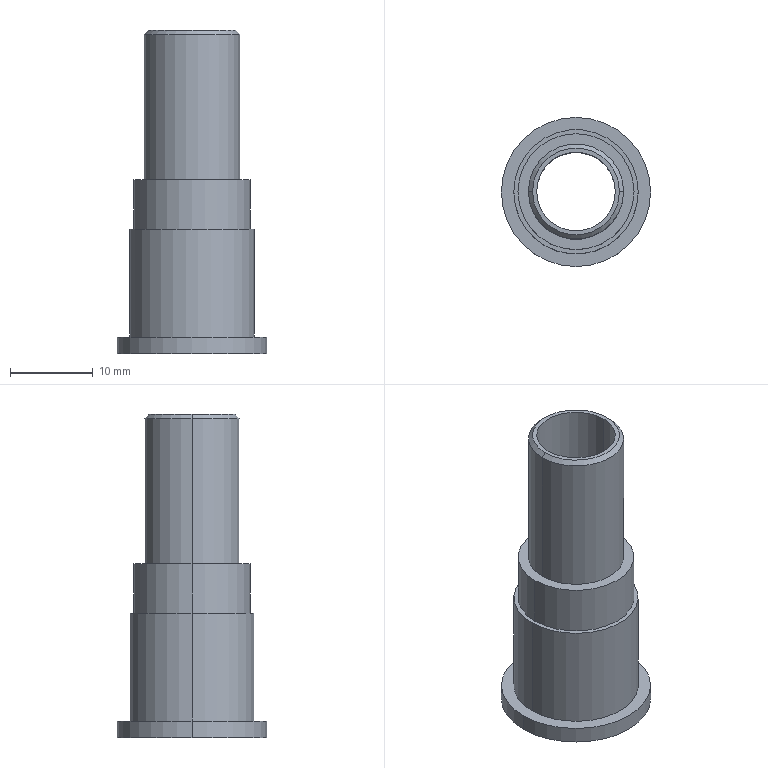Part | SolidWorks | features ICE 4, Chamfer 2, Extrusion 1 | 1 solid | 19 faces | box 18 x 18 x 39 mm | volume 2785 mm3 | cylinder 10 | plane 5 | cone 4 | commonest cylinder face diameters 9.5 x2 11.5 x2 14 x2 15 x2 18 x2
STEP:
#1=CARTESIAN_POINT('',(4.75,0.,10.));
#2=VERTEX_POINT('',#1);
#3=CARTESIAN_POINT('',(-4.75,0.,10.));
#4=VERTEX_POINT('',#3);
#5=CARTESIAN_POINT('',(0.,0.,10.));
#6=DIRECTION('',(0.,0.,-1.));
#7=DIRECTION('',(1.,0.,0.));
#8=AXIS2_PLACEMENT_3D('',#5,#6,#7);
#9=CIRCLE('',#8,4.75);
#10=EDGE_CURVE('',#2,#4,#9,.T.);
#11=ORIENTED_EDGE('',*,*,#10,.F.);
#12=CARTESIAN_POINT('',(5.05,0.,0.));
#13=VERTEX_POINT('',#12);
#14=CARTESIAN_POINT('',(4.75,0.,10.));
#15=DIRECTION('',(0.02999,0.,-0.9996));
#16=VECTOR('',#15,1000.);
#17=LINE('',#14,#16);
#18=EDGE_CURVE('',#2,#13,#17,.T.);
#19=ORIENTED_EDGE('',*,*,#18,.T.);
#20=CARTESIAN_POINT('',(-5.05,0.,0.));
#21=VERTEX_POINT('',#20);
#22=CARTESIAN_POINT('',(0.,0.,0.));
#23=DIRECTION('',(0.,0.,1.));
#24=DIRECTION('',(1.,0.,0.));
#25=AXIS2_PLACEMENT_3D('',#22,#23,#24);
#26=CIRCLE('',#25,5.05);
#27=EDGE_CURVE('',#21,#13,#26,.T.);
#28=ORIENTED_EDGE('',*,*,#27,.F.);
#29=CARTESIAN_POINT('',(-4.75,0.,10.));
#30=DIRECTION('',(-0.02999,0.,-0.9996));
#31=VECTOR('',#30,1000.);
#32=LINE('',#29,#31);
#33=EDGE_CURVE('',#4,#21,#32,.T.);
#34=ORIENTED_EDGE('',*,*,#33,.F.);
#35=EDGE_LOOP('',(#11,#19,#28,#34));
#36=FACE_OUTER_BOUND('',#35,.T.);
#37=CARTESIAN_POINT('',(0.,0.,10.));
#38=DIRECTION('',(0.,0.,-1.));
#39=DIRECTION('',(-1.,0.,0.));
#40=AXIS2_PLACEMENT_3D('',#37,#38,#39);
#41=CONICAL_SURFACE('',#40,4.75,0.02999);
#42=ADVANCED_FACE('',(#36),#41,.F.);
#43=CARTESIAN_POINT('',(5.25,0.,39.));
#44=VERTEX_POINT('',#43);
#45=CARTESIAN_POINT('',(-5.25,0.,39.));
#46=VERTEX_POINT('',#45);
#47=CARTESIAN_POINT('',(0.,0.,39.));
#48=DIRECTION('',(0.,0.,1.));
#49=DIRECTION('',(1.,0.,0.));
#50=AXIS2_PLACEMENT_3D('',#47,#48,#49);
#51=CIRCLE('',#50,5.25);
#52=EDGE_CURVE('',#44,#46,#51,.T.);
#53=ORIENTED_EDGE('',*,*,#52,.F.);
#54=CARTESIAN_POINT('',(5.75,0.,38.5));
#55=VERTEX_POINT('',#54);
#56=CARTESIAN_POINT('',(5.25,0.,39.));
#57=DIRECTION('',(0.7071,0.,-0.7071));
#58=VECTOR('',#57,1000.);
#59=LINE('',#56,#58);
#60=EDGE_CURVE('',#44,#55,#59,.T.);
#61=ORIENTED_EDGE('',*,*,#60,.T.);
#62=CARTESIAN_POINT('',(-5.75,0.,38.5));
#63=VERTEX_POINT('',#62);
#64=CARTESIAN_POINT('',(0.,0.,38.5));
#65=DIRECTION('',(0.,0.,-1.));
#66=DIRECTION('',(1.,0.,0.));
#67=AXIS2_PLACEMENT_3D('',#64,#65,#66);
#68=CIRCLE('',#67,5.75);
#69=EDGE_CURVE('',#63,#55,#68,.T.);
#70=ORIENTED_EDGE('',*,*,#69,.F.);
#71=CARTESIAN_POINT('',(-5.25,0.,39.));
#72=DIRECTION('',(-0.7071,0.,-0.7071));
#73=VECTOR('',#72,1000.);
#74=LINE('',#71,#73);
#75=EDGE_CURVE('',#46,#63,#74,.T.);
#76=ORIENTED_EDGE('',*,*,#75,.F.);
#77=EDGE_LOOP('',(#53,#61,#70,#76));
#78=FACE_OUTER_BOUND('',#77,.T.);
#79=CARTESIAN_POINT('',(0.,0.,39.));
#80=DIRECTION('',(0.,0.,-1.));
#81=DIRECTION('',(-1.,0.,0.));
#82=AXIS2_PLACEMENT_3D('',#79,#80,#81);
#83=CONICAL_SURFACE('',#82,5.25,0.7854);
#84=ADVANCED_FACE('',(#78),#83,.T.);
#85=CARTESIAN_POINT('',(4.75,0.,39.));
#86=VERTEX_POINT('',#85);
#87=CARTESIAN_POINT('',(-4.75,0.,39.));
#88=VERTEX_POINT('',#87);
#89=CARTESIAN_POINT('',(0.,0.,39.));
#90=DIRECTION('',(0.,0.,-1.));
#91=DIRECTION('',(-1.,0.,0.));
#92=AXIS2_PLACEMENT_3D('',#89,#90,#91);
#93=CIRCLE('',#92,4.75);
#94=EDGE_CURVE('',#86,#88,#93,.T.);
#95=ORIENTED_EDGE('',*,*,#94,.F.);
#96=CARTESIAN_POINT('',(4.75,0.,39.));
#97=DIRECTION('',(0.,0.,-1.));
#98=VECTOR('',#97,1000.);
#99=LINE('',#96,#98);
#100=EDGE_CURVE('',#86,#2,#99,.T.);
#101=ORIENTED_EDGE('',*,*,#100,.T.);
#102=ORIENTED_EDGE('',*,*,#10,.T.);
#103=CARTESIAN_POINT('',(-4.75,0.,39.));
#104=DIRECTION('',(0.,0.,-1.));
#105=VECTOR('',#104,1000.);
#106=LINE('',#103,#105);
#107=EDGE_CURVE('',#88,#4,#106,.T.);
#108=ORIENTED_EDGE('',*,*,#107,.F.);
#109=EDGE_LOOP('',(#95,#101,#102,#108));
#110=FACE_OUTER_BOUND('',#109,.T.);
#111=CARTESIAN_POINT('',(0.,0.,39.));
#112=DIRECTION('',(0.,0.,-1.));
#113=DIRECTION('',(-1.,0.,0.));
#114=AXIS2_PLACEMENT_3D('',#111,#112,#113);
#115=CYLINDRICAL_SURFACE('',#114,4.75);
#116=ADVANCED_FACE('',(#110),#115,.F.);
#117=ORIENTED_EDGE('',*,*,#69,.T.);
#118=CARTESIAN_POINT('',(5.75,0.,21.));
#119=VERTEX_POINT('',#118);
#120=CARTESIAN_POINT('',(5.75,0.,39.));
#121=DIRECTION('',(0.,0.,-1.));
#122=VECTOR('',#121,1000.);
#123=LINE('',#120,#122);
#124=EDGE_CURVE('',#55,#119,#123,.T.);
#125=ORIENTED_EDGE('',*,*,#124,.T.);
#126=CARTESIAN_POINT('',(-5.75,0.,21.));
#127=VERTEX_POINT('',#126);
#128=CARTESIAN_POINT('',(0.,0.,21.));
#129=DIRECTION('',(0.,0.,1.));
#130=DIRECTION('',(1.,0.,0.));
#131=AXIS2_PLACEMENT_3D('',#128,#129,#130);
#132=CIRCLE('',#131,5.75);
#133=EDGE_CURVE('',#119,#127,#132,.T.);
#134=ORIENTED_EDGE('',*,*,#133,.T.);
#135=CARTESIAN_POINT('',(-5.75,0.,39.));
#136=DIRECTION('',(0.,0.,-1.));
#137=VECTOR('',#136,1000.);
#138=LINE('',#135,#137);
#139=EDGE_CURVE('',#63,#127,#138,.T.);
#140=ORIENTED_EDGE('',*,*,#139,.F.);
#141=EDGE_LOOP('',(#117,#125,#134,#140));
#142=FACE_OUTER_BOUND('',#141,.T.);
#143=CARTESIAN_POINT('',(0.,0.,39.));
#144=DIRECTION('',(0.,0.,-1.));
#145=DIRECTION('',(-1.,0.,0.));
#146=AXIS2_PLACEMENT_3D('',#143,#144,#145);
#147=CYLINDRICAL_SURFACE('',#146,5.75);
#148=ADVANCED_FACE('',(#142),#147,.T.);
#149=CARTESIAN_POINT('',(7.,0.,21.));
#150=VERTEX_POINT('',#149);
#151=CARTESIAN_POINT('',(-7.,0.,21.));
#152=VERTEX_POINT('',#151);
#153=CARTESIAN_POINT('',(0.,0.,21.));
#154=DIRECTION('',(0.,0.,1.));
#155=DIRECTION('',(1.,0.,0.));
#156=AXIS2_PLACEMENT_3D('',#153,#154,#155);
#157=CIRCLE('',#156,7.);
#158=EDGE_CURVE('',#150,#152,#157,.T.);
#159=ORIENTED_EDGE('',*,*,#158,.F.);
#160=CARTESIAN_POINT('',(7.,0.,15.));
#161=VERTEX_POINT('',#160);
#162=CARTESIAN_POINT('',(7.,0.,21.));
#163=DIRECTION('',(0.,0.,-1.));
#164=VECTOR('',#163,1000.);
#165=LINE('',#162,#164);
#166=EDGE_CURVE('',#150,#161,#165,.T.);
#167=ORIENTED_EDGE('',*,*,#166,.T.);
#168=CARTESIAN_POINT('',(-7.,0.,15.));
#169=VERTEX_POINT('',#168);
#170=CARTESIAN_POINT('',(0.,0.,15.));
#171=DIRECTION('',(0.,0.,1.));
#172=DIRECTION('',(1.,0.,0.));
#173=AXIS2_PLACEMENT_3D('',#170,#171,#172);
#174=CIRCLE('',#173,7.);
#175=EDGE_CURVE('',#161,#169,#174,.T.);
#176=ORIENTED_EDGE('',*,*,#175,.T.);
#177=CARTESIAN_POINT('',(-7.,0.,21.));
#178=DIRECTION('',(0.,0.,-1.));
#179=VECTOR('',#178,1000.);
#180=LINE('',#177,#179);
#181=EDGE_CURVE('',#152,#169,#180,.T.);
#182=ORIENTED_EDGE('',*,*,#181,.F.);
#183=EDGE_LOOP('',(#159,#167,#176,#182));
#184=FACE_OUTER_BOUND('',#183,.T.);
#185=CARTESIAN_POINT('',(0.,0.,21.));
#186=DIRECTION('',(0.,0.,-1.));
#187=DIRECTION('',(-1.,0.,0.));
#188=AXIS2_PLACEMENT_3D('',#185,#186,#187);
#189=CYLINDRICAL_SURFACE('',#188,7.);
#190=ADVANCED_FACE('',(#184),#189,.T.);
#191=CARTESIAN_POINT('',(7.5,0.,15.));
#192=VERTEX_POINT('',#191);
#193=CARTESIAN_POINT('',(-7.5,0.,15.));
#194=VERTEX_POINT('',#193);
#195=CARTESIAN_POINT('',(0.,0.,15.));
#196=DIRECTION('',(0.,0.,1.));
#197=DIRECTION('',(1.,0.,0.));
#198=AXIS2_PLACEMENT_3D('',#195,#196,#197);
#199=CIRCLE('',#198,7.5);
#200=EDGE_CURVE('',#192,#194,#199,.T.);
#201=ORIENTED_EDGE('',*,*,#200,.F.);
#202=CARTESIAN_POINT('',(7.5,0.,2.));
#203=VERTEX_POINT('',#202);
#204=CARTESIAN_POINT('',(7.5,0.,15.));
#205=DIRECTION('',(0.,0.,-1.));
#206=VECTOR('',#205,1000.);
#207=LINE('',#204,#206);
#208=EDGE_CURVE('',#192,#203,#207,.T.);
#209=ORIENTED_EDGE('',*,*,#208,.T.);
#210=CARTESIAN_POINT('',(-7.5,0.,2.));
#211=VERTEX_POINT('',#210);
#212=CARTESIAN_POINT('',(0.,0.,2.));
#213=DIRECTION('',(0.,0.,1.));
#214=DIRECTION('',(1.,0.,0.));
#215=AXIS2_PLACEMENT_3D('',#212,#213,#214);
#216=CIRCLE('',#215,7.5);
#217=EDGE_CURVE('',#203,#211,#216,.T.);
#218=ORIENTED_EDGE('',*,*,#217,.T.);
#219=CARTESIAN_POINT('',(-7.5,0.,15.));
#220=DIRECTION('',(0.,0.,-1.));
#221=VECTOR('',#220,1000.);
#222=LINE('',#219,#221);
#223=EDGE_CURVE('',#194,#211,#222,.T.);
#224=ORIENTED_EDGE('',*,*,#223,.F.);
#225=EDGE_LOOP('',(#201,#209,#218,#224));
#226=FACE_OUTER_BOUND('',#225,.T.);
#227=CARTESIAN_POINT('',(0.,0.,15.));
#228=DIRECTION('',(0.,0.,-1.));
#229=DIRECTION('',(-1.,0.,0.));
#230=AXIS2_PLACEMENT_3D('',#227,#228,#229);
#231=CYLINDRICAL_SURFACE('',#230,7.5);
#232=ADVANCED_FACE('',(#226),#231,.T.);
#233=CARTESIAN_POINT('',(9.,0.,2.));
#234=VERTEX_POINT('',#233);
#235=CARTESIAN_POINT('',(-9.,0.,2.));
#236=VERTEX_POINT('',#235);
#237=CARTESIAN_POINT('',(0.,0.,2.));
#238=DIRECTION('',(0.,0.,1.));
#239=DIRECTION('',(1.,0.,0.));
#240=AXIS2_PLACEMENT_3D('',#237,#238,#239);
#241=CIRCLE('',#240,9.);
#242=EDGE_CURVE('',#234,#236,#241,.T.);
#243=ORIENTED_EDGE('',*,*,#242,.F.);
#244=CARTESIAN_POINT('',(9.,0.,0.));
#245=VERTEX_POINT('',#244);
#246=CARTESIAN_POINT('',(9.,0.,2.));
#247=DIRECTION('',(0.,0.,-1.));
#248=VECTOR('',#247,1000.);
#249=LINE('',#246,#248);
#250=EDGE_CURVE('',#234,#245,#249,.T.);
#251=ORIENTED_EDGE('',*,*,#250,.T.);
#252=CARTESIAN_POINT('',(-9.,0.,0.));
#253=VERTEX_POINT('',#252);
#254=CARTESIAN_POINT('',(0.,0.,0.));
#255=DIRECTION('',(0.,0.,1.));
#256=DIRECTION('',(1.,0.,0.));
#257=AXIS2_PLACEMENT_3D('',#254,#255,#256);
#258=CIRCLE('',#257,9.);
#259=EDGE_CURVE('',#245,#253,#258,.T.);
#260=ORIENTED_EDGE('',*,*,#259,.T.);
#261=CARTESIAN_POINT('',(-9.,0.,2.));
#262=DIRECTION('',(0.,0.,-1.));
#263=VECTOR('',#262,1000.);
#264=LINE('',#261,#263);
#265=EDGE_CURVE('',#236,#253,#264,.T.);
#266=ORIENTED_EDGE('',*,*,#265,.F.);
#267=EDGE_LOOP('',(#243,#251,#260,#266));
#268=FACE_OUTER_BOUND('',#267,.T.);
#269=CARTESIAN_POINT('',(0.,0.,2.));
#270=DIRECTION('',(0.,0.,-1.));
#271=DIRECTION('',(-1.,0.,0.));
#272=AXIS2_PLACEMENT_3D('',#269,#270,#271);
#273=CYLINDRICAL_SURFACE('',#272,9.);
#274=ADVANCED_FACE('',(#268),#273,.T.);
#275=CARTESIAN_POINT('',(0.,0.,21.));
#276=DIRECTION('',(0.,0.,1.));
#277=DIRECTION('',(1.,0.,0.));
#278=AXIS2_PLACEMENT_3D('',#275,#276,#277);
#279=CIRCLE('',#278,7.);
#280=EDGE_CURVE('',#152,#150,#279,.T.);
#281=ORIENTED_EDGE('',*,*,#280,.T.);
#282=ORIENTED_EDGE('',*,*,#158,.T.);
#283=EDGE_LOOP('',(#281,#282));
#284=FACE_OUTER_BOUND('',#283,.T.);
#285=CARTESIAN_POINT('',(0.,0.,21.));
#286=DIRECTION('',(0.,0.,1.));
#287=DIRECTION('',(1.,0.,0.));
#288=AXIS2_PLACEMENT_3D('',#285,#286,#287);
#289=CIRCLE('',#288,5.75);
#290=EDGE_CURVE('',#127,#119,#289,.T.);
#291=ORIENTED_EDGE('',*,*,#290,.F.);
#292=ORIENTED_EDGE('',*,*,#133,.F.);
#293=EDGE_LOOP('',(#291,#292));
#294=FACE_BOUND('',#293,.T.);
#295=CARTESIAN_POINT('',(0.,0.,21.));
#296=DIRECTION('',(0.,0.,1.));
#297=DIRECTION('',(1.,0.,0.));
#298=AXIS2_PLACEMENT_3D('',#295,#296,#297);
#299=PLANE('',#298);
#300=ADVANCED_FACE('',(#284,#294),#299,.T.);
#301=CARTESIAN_POINT('',(0.,0.,15.));
#302=DIRECTION('',(0.,0.,1.));
#303=DIRECTION('',(1.,0.,0.));
#304=AXIS2_PLACEMENT_3D('',#301,#302,#303);
#305=CIRCLE('',#304,7.5);
#306=EDGE_CURVE('',#194,#192,#305,.T.);
#307=ORIENTED_EDGE('',*,*,#306,.T.);
#308=ORIENTED_EDGE('',*,*,#200,.T.);
#309=EDGE_LOOP('',(#307,#308));
#310=FACE_OUTER_BOUND('',#309,.T.);
#311=CARTESIAN_POINT('',(0.,0.,15.));
#312=DIRECTION('',(0.,0.,1.));
#313=DIRECTION('',(1.,0.,0.));
#314=AXIS2_PLACEMENT_3D('',#311,#312,#313);
#315=CIRCLE('',#314,7.);
#316=EDGE_CURVE('',#169,#161,#315,.T.);
#317=ORIENTED_EDGE('',*,*,#316,.F.);
#318=ORIENTED_EDGE('',*,*,#175,.F.);
#319=EDGE_LOOP('',(#317,#318));
#320=FACE_BOUND('',#319,.T.);
#321=CARTESIAN_POINT('',(0.,0.,15.));
#322=DIRECTION('',(0.,0.,1.));
#323=DIRECTION('',(1.,0.,0.));
#324=AXIS2_PLACEMENT_3D('',#321,#322,#323);
#325=PLANE('',#324);
#326=ADVANCED_FACE('',(#310,#320),#325,.T.);
#327=CARTESIAN_POINT('',(0.,0.,2.));
#328=DIRECTION('',(0.,0.,1.));
#329=DIRECTION('',(1.,0.,0.));
#330=AXIS2_PLACEMENT_3D('',#327,#328,#329);
#331=CIRCLE('',#330,9.);
#332=EDGE_CURVE('',#236,#234,#331,.T.);
#333=ORIENTED_EDGE('',*,*,#332,.T.);
#334=ORIENTED_EDGE('',*,*,#242,.T.);
#335=EDGE_LOOP('',(#333,#334));
#336=FACE_OUTER_BOUND('',#335,.T.);
#337=CARTESIAN_POINT('',(0.,0.,2.));
#338=DIRECTION('',(0.,0.,1.));
#339=DIRECTION('',(1.,0.,0.));
#340=AXIS2_PLACEMENT_3D('',#337,#338,#339);
#341=CIRCLE('',#340,7.5);
#342=EDGE_CURVE('',#211,#203,#341,.T.);
#343=ORIENTED_EDGE('',*,*,#342,.F.);
#344=ORIENTED_EDGE('',*,*,#217,.F.);
#345=EDGE_LOOP('',(#343,#344));
#346=FACE_BOUND('',#345,.T.);
#347=CARTESIAN_POINT('',(0.,0.,2.));
#348=DIRECTION('',(0.,0.,1.));
#349=DIRECTION('',(1.,0.,0.));
#350=AXIS2_PLACEMENT_3D('',#347,#348,#349);
#351=PLANE('',#350);
#352=ADVANCED_FACE('',(#336,#346),#351,.T.);
#353=ORIENTED_EDGE('',*,*,#250,.F.);
#354=ORIENTED_EDGE('',*,*,#332,.F.);
#355=ORIENTED_EDGE('',*,*,#265,.T.);
#356=CARTESIAN_POINT('',(0.,0.,0.));
#357=DIRECTION('',(0.,0.,1.));
#358=DIRECTION('',(1.,0.,0.));
#359=AXIS2_PLACEMENT_3D('',#356,#357,#358);
#360=CIRCLE('',#359,9.);
#361=EDGE_CURVE('',#253,#245,#360,.T.);
#362=ORIENTED_EDGE('',*,*,#361,.T.);
#363=EDGE_LOOP('',(#353,#354,#355,#362));
#364=FACE_OUTER_BOUND('',#363,.T.);
#365=CARTESIAN_POINT('',(0.,0.,2.));
#366=DIRECTION('',(0.,0.,-1.));
#367=DIRECTION('',(-1.,0.,0.));
#368=AXIS2_PLACEMENT_3D('',#365,#366,#367);
#369=CYLINDRICAL_SURFACE('',#368,9.);
#370=ADVANCED_FACE('',(#364),#369,.T.);
#371=ORIENTED_EDGE('',*,*,#27,.T.);
#372=CARTESIAN_POINT('',(0.,0.,0.));
#373=DIRECTION('',(0.,0.,1.));
#374=DIRECTION('',(1.,0.,0.));
#375=AXIS2_PLACEMENT_3D('',#372,#373,#374);
#376=CIRCLE('',#375,5.05);
#377=EDGE_CURVE('',#13,#21,#376,.T.);
#378=ORIENTED_EDGE('',*,*,#377,.T.);
#379=EDGE_LOOP('',(#371,#378));
#380=FACE_BOUND('',#379,.T.);
#381=ORIENTED_EDGE('',*,*,#361,.F.);
#382=ORIENTED_EDGE('',*,*,#259,.F.);
#383=EDGE_LOOP('',(#381,#382));
#384=FACE_OUTER_BOUND('',#383,.T.);
#385=CARTESIAN_POINT('',(0.,0.,0.));
#386=DIRECTION('',(0.,0.,1.));
#387=DIRECTION('',(1.,0.,0.));
#388=AXIS2_PLACEMENT_3D('',#385,#386,#387);
#389=PLANE('',#388);
#390=ADVANCED_FACE('',(#380,#384),#389,.F.);
#391=ORIENTED_EDGE('',*,*,#208,.F.);
#392=ORIENTED_EDGE('',*,*,#306,.F.);
#393=ORIENTED_EDGE('',*,*,#223,.T.);
#394=ORIENTED_EDGE('',*,*,#342,.T.);
#395=EDGE_LOOP('',(#391,#392,#393,#394));
#396=FACE_OUTER_BOUND('',#395,.T.);
#397=CARTESIAN_POINT('',(0.,0.,15.));
#398=DIRECTION('',(0.,0.,-1.));
#399=DIRECTION('',(-1.,0.,0.));
#400=AXIS2_PLACEMENT_3D('',#397,#398,#399);
#401=CYLINDRICAL_SURFACE('',#400,7.5);
#402=ADVANCED_FACE('',(#396),#401,.T.);
#403=ORIENTED_EDGE('',*,*,#166,.F.);
#404=ORIENTED_EDGE('',*,*,#280,.F.);
#405=ORIENTED_EDGE('',*,*,#181,.T.);
#406=ORIENTED_EDGE('',*,*,#316,.T.);
#407=EDGE_LOOP('',(#403,#404,#405,#406));
#408=FACE_OUTER_BOUND('',#407,.T.);
#409=CARTESIAN_POINT('',(0.,0.,21.));
#410=DIRECTION('',(0.,0.,-1.));
#411=DIRECTION('',(-1.,0.,0.));
#412=AXIS2_PLACEMENT_3D('',#409,#410,#411);
#413=CYLINDRICAL_SURFACE('',#412,7.);
#414=ADVANCED_FACE('',(#408),#413,.T.);
#415=ORIENTED_EDGE('',*,*,#124,.F.);
#416=CARTESIAN_POINT('',(0.,0.,38.5));
#417=DIRECTION('',(0.,0.,-1.));
#418=DIRECTION('',(1.,0.,0.));
#419=AXIS2_PLACEMENT_3D('',#416,#417,#418);
#420=CIRCLE('',#419,5.75);
#421=EDGE_CURVE('',#55,#63,#420,.T.);
#422=ORIENTED_EDGE('',*,*,#421,.T.);
#423=ORIENTED_EDGE('',*,*,#139,.T.);
#424=ORIENTED_EDGE('',*,*,#290,.T.);
#425=EDGE_LOOP('',(#415,#422,#423,#424));
#426=FACE_OUTER_BOUND('',#425,.T.);
#427=CARTESIAN_POINT('',(0.,0.,39.));
#428=DIRECTION('',(0.,0.,-1.));
#429=DIRECTION('',(-1.,0.,0.));
#430=AXIS2_PLACEMENT_3D('',#427,#428,#429);
#431=CYLINDRICAL_SURFACE('',#430,5.75);
#432=ADVANCED_FACE('',(#426),#431,.T.);
#433=CARTESIAN_POINT('',(0.,0.,39.));
#434=DIRECTION('',(0.,0.,1.));
#435=DIRECTION('',(1.,0.,0.));
#436=AXIS2_PLACEMENT_3D('',#433,#434,#435);
#437=CIRCLE('',#436,5.25);
#438=EDGE_CURVE('',#46,#44,#437,.T.);
#439=ORIENTED_EDGE('',*,*,#438,.T.);
#440=ORIENTED_EDGE('',*,*,#52,.T.);
#441=EDGE_LOOP('',(#439,#440));
#442=FACE_OUTER_BOUND('',#441,.T.);
#443=CARTESIAN_POINT('',(0.,0.,39.));
#444=DIRECTION('',(0.,0.,-1.));
#445=DIRECTION('',(-1.,0.,0.));
#446=AXIS2_PLACEMENT_3D('',#443,#444,#445);
#447=CIRCLE('',#446,4.75);
#448=EDGE_CURVE('',#88,#86,#447,.T.);
#449=ORIENTED_EDGE('',*,*,#448,.T.);
#450=ORIENTED_EDGE('',*,*,#94,.T.);
#451=EDGE_LOOP('',(#449,#450));
#452=FACE_BOUND('',#451,.T.);
#453=CARTESIAN_POINT('',(0.,0.,39.));
#454=DIRECTION('',(0.,0.,1.));
#455=DIRECTION('',(1.,0.,0.));
#456=AXIS2_PLACEMENT_3D('',#453,#454,#455);
#457=PLANE('',#456);
#458=ADVANCED_FACE('',(#442,#452),#457,.T.);
#459=ORIENTED_EDGE('',*,*,#100,.F.);
#460=ORIENTED_EDGE('',*,*,#448,.F.);
#461=ORIENTED_EDGE('',*,*,#107,.T.);
#462=CARTESIAN_POINT('',(0.,0.,10.));
#463=DIRECTION('',(0.,0.,-1.));
#464=DIRECTION('',(1.,0.,0.));
#465=AXIS2_PLACEMENT_3D('',#462,#463,#464);
#466=CIRCLE('',#465,4.75);
#467=EDGE_CURVE('',#4,#2,#466,.T.);
#468=ORIENTED_EDGE('',*,*,#467,.T.);
#469=EDGE_LOOP('',(#459,#460,#461,#468));
#470=FACE_OUTER_BOUND('',#469,.T.);
#471=CARTESIAN_POINT('',(0.,0.,39.));
#472=DIRECTION('',(0.,0.,-1.));
#473=DIRECTION('',(-1.,0.,0.));
#474=AXIS2_PLACEMENT_3D('',#471,#472,#473);
#475=CYLINDRICAL_SURFACE('',#474,4.75);
#476=ADVANCED_FACE('',(#470),#475,.F.);
#477=ORIENTED_EDGE('',*,*,#60,.F.);
#478=ORIENTED_EDGE('',*,*,#438,.F.);
#479=ORIENTED_EDGE('',*,*,#75,.T.);
#480=ORIENTED_EDGE('',*,*,#421,.F.);
#481=EDGE_LOOP('',(#477,#478,#479,#480));
#482=FACE_OUTER_BOUND('',#481,.T.);
#483=CARTESIAN_POINT('',(0.,0.,39.));
#484=DIRECTION('',(0.,0.,-1.));
#485=DIRECTION('',(-1.,0.,0.));
#486=AXIS2_PLACEMENT_3D('',#483,#484,#485);
#487=CONICAL_SURFACE('',#486,5.25,0.7854);
#488=ADVANCED_FACE('',(#482),#487,.T.);
#489=ORIENTED_EDGE('',*,*,#18,.F.);
#490=ORIENTED_EDGE('',*,*,#467,.F.);
#491=ORIENTED_EDGE('',*,*,#33,.T.);
#492=ORIENTED_EDGE('',*,*,#377,.F.);
#493=EDGE_LOOP('',(#489,#490,#491,#492));
#494=FACE_OUTER_BOUND('',#493,.T.);
#495=CARTESIAN_POINT('',(0.,0.,10.));
#496=DIRECTION('',(0.,0.,-1.));
#497=DIRECTION('',(-1.,0.,0.));
#498=AXIS2_PLACEMENT_3D('',#495,#496,#497);
#499=CONICAL_SURFACE('',#498,4.75,0.02999);
#500=ADVANCED_FACE('',(#494),#499,.F.);
#501=CLOSED_SHELL('',(#42,#84,#116,#148,#190,#232,#274,#300,#326,#352,#370,#390,#402,#414,#432,#458,#476,#488,#500));
#502=MANIFOLD_SOLID_BREP('',#501);
#503=CARTESIAN_POINT('',(0.,0.,0.));
#504=DIRECTION('',(0.,0.,1.));
#505=DIRECTION('',(1.,0.,0.));
#506=AXIS2_PLACEMENT_3D('',#503,#504,#505);
#507=(LENGTH_UNIT()NAMED_UNIT(*)SI_UNIT(.MILLI.,.METRE.));
#508=UNCERTAINTY_MEASURE_WITH_UNIT(LENGTH_MEASURE(0.00001),#507,'','');
#509=(NAMED_UNIT(*)PLANE_ANGLE_UNIT()SI_UNIT($,.RADIAN.));
#510=(NAMED_UNIT(*)SI_UNIT($,.STERADIAN.)SOLID_ANGLE_UNIT());
#511=(GEOMETRIC_REPRESENTATION_CONTEXT(3)GLOBAL_UNCERTAINTY_ASSIGNED_CONTEXT((#508))GLOBAL_UNIT_ASSIGNED_CONTEXT((#507,#509,#510))REPRESENTATION_CONTEXT('',''));
#512=ADVANCED_BREP_SHAPE_REPRESENTATION('',(#502,#506),#511);